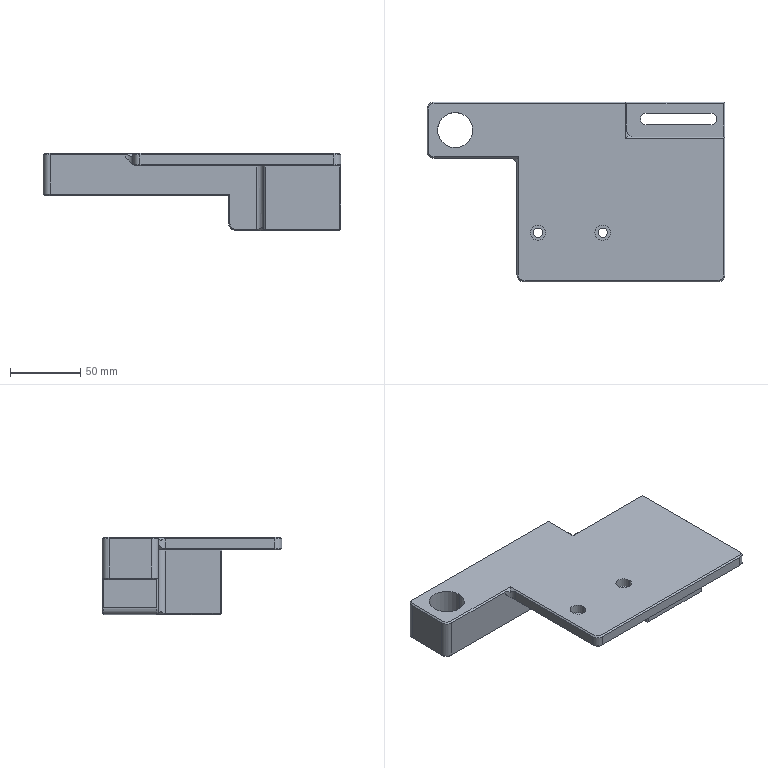NC program | NX | posted with a generic post | part box 212 x 128 x 55 mm
Lines 7214 to 7327 of 7327:
(ZLEVEL_PROFILE_1_COPY_1_COPY_COPY_1_COPY_COPY , TOOL : D8A45)
N14360 T06 M6
N14362 G54
N14364 G17 G0 G90 X-102.326 Y67.497 S6500 M3
N14366 G43 Z30. H6
N14368 Z-2.
N14370 G94 G1 Z-3. F1000.
N14372 X-101.693 Y66.4
N14374 G3 X-101. Y66. R0.8
N14376 G1 X35.001
N14378 X35.735 Y65.989
N14380 G2 X37.997 Y63.615 R2.506
N14382 G1 X38. Y63.002
N14384 Y41.
N14386 X105.001
N14388 X105.502 Y40.998
N14390 G2 X108. Y38.49 R2.508
N14392 G1 Y-59.
N14394 G2 X101. Y-66. R7.
N14396 G1 X-37.
N14398 G2 X-44. Y-59. R7.
N14400 G1 Y21.997
N14402 X-44.12 Y22.
N14404 X-101.
N14406 G2 X-108. Y29. R7.
N14408 G1 Y59.
N14410 G2 X-101. Y66. R7.
N14412 G3 X-100.307 Y66.4 R0.8
N14414 G1 X-99.614 Y67.6
N14416 Z-2.
N14418 G0 Z30.
(ZLEVEL_PROFILE_1_COPY_1_COPY_COPY_1_COPY_COPY_COPY_1 , TOOL : D8A45)
N14420 X-95.877 Y45.446
N14422 Z0.
N14424 G1 Z-1.
N14426 X-97.183 Y44.693
N14428 G3 X-97.583 Y44. R0.8
N14430 G1 Y43.992
N14432 G3 X-85.992 Y32.417 R11.583
N14434 X-97.583 Y44. R-11.583
N14436 X-97.183 Y43.307 R0.8
N14438 G1 X-95.877 Y42.554
N14440 Z0.
N14442 G0 Z30.
N14444 X17.312 Y-31.459
N14446 Z0.
N14448 G1 Z-1.
N14450 X18.307 Y-33.183
N14452 G3 X19. Y-33.583 R0.8
N14454 X23.583 Y-29. R4.583
N14456 X19. Y-33.583 R-4.583
N14458 X19.693 Y-33.183 R0.8
N14460 G1 X20.688 Y-31.459
N14462 Z0.
N14464 G0 Z30.
N14466 X-28.688
N14468 Z0.
N14470 G1 Z-1.
N14472 X-27.693 Y-33.183
N14474 G3 X-27. Y-33.583 R0.8
N14476 X-22.417 Y-29. R4.583
N14478 X-27. Y-33.583 R-4.583
N14480 X-26.307 Y-33.183 R0.8
N14482 G1 X-25.312 Y-31.459
N14484 Z0.
N14486 G0 Z30.
(ZLEVEL_PROFILE_1_COPY_1_COPY_COPY_1_COPY_COPY_COPY_1_COPY , TOOL : D8A45)
N14488 X40.29 Y66.6
N14490 Z-38.
N14492 G1 Z-39.
N14494 X39.345 Y65.4
N14496 G3 X40.038 Y65. R0.8
N14498 G1 X105.001
N14500 X105.516 Y64.997
N14502 G2 X106.996 Y63.517 R1.49
N14504 G1 X107. Y63.002
N14506 Y43.039
N14508 G3 X107.4 Y42.346 R0.8
N14510 G1 X108.6 Y43.29
N14512 Z-38.
N14514 G0 Z30.
N14516 M5
(刀补12 , TOOL : D10)
N14518 T09 M6
N14520 G54
N14522 G17 G0 G90 X-86. Y44. S5000 M3
N14524 G43 Z30. H9
N14526 Z0.5
N14528 G41 G94 G1 X-82.374 Y41.508 F1000. D9
N14530 G3 X-78.5 Y44. R2.738
N14532 X-78.5 Y44. Z-3.5 I-7.5 J0.
N14534 X-78.5 Y44. Z-7.5 I-7.5 J0.
N14536 X-78.5 Y44. Z-11.5 I-7.5 J0.
N14538 X-78.5 Y44. Z-15.5 I-7.5 J0.
N14540 X-78.5 Y44. Z-19.5 I-7.5 J0.
N14542 X-78.5 Y44. Z-23.5 I-7.5 J0.
N14544 X-78.5 Y44. Z-27.5 I-7.5 J0.
N14546 X-91.303 Y38.697 Z-30. R-7.5
N14548 X-80.697 Y38.697 R7.5
N14550 X-91.303 Y38.697 R-7.5
N14552 X-86.802 Y39.674 R2.738
N14554 G40
N14556 G1 X-86. Y44.
N14558 G0 Z30.
N14560 M5
N14562 M2